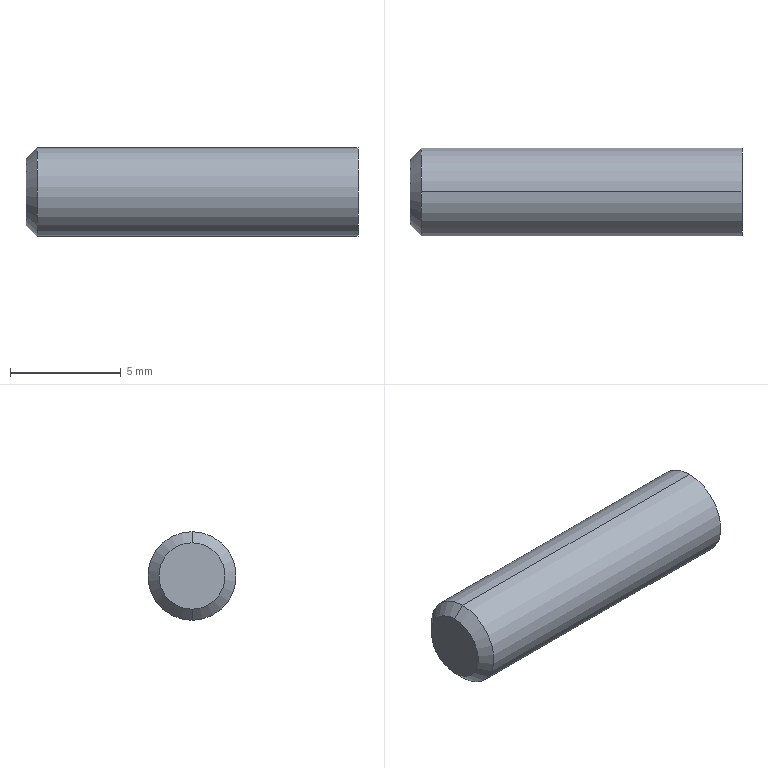Part | STEP file | 1 solid | 6 faces | box 15 x 4 x 4 mm | volume 187.056 mm3 | cylinder 2 | cone 2 | plane 2 | commonest cylinder face diameters 4 x2
STEP:
#1=CARTESIAN_POINT('',(0.,0.,0.));
#2=DIRECTION('',(0.,0.,1.));
#3=DIRECTION('',(1.,0.,0.));
#4=AXIS2_PLACEMENT_3D('',#1,#2,#3);
#5=CARTESIAN_POINT('',(-516.273,4552.173,1399.094));
#6=VERTEX_POINT('',#5);
#7=CARTESIAN_POINT('',(-501.773,4552.173,1399.094));
#8=VERTEX_POINT('',#7);
#9=CARTESIAN_POINT('',(-516.273,4552.173,1399.094));
#10=DIRECTION('',(1.,0.,0.));
#11=VECTOR('',#10,1.);
#12=LINE('',#9,#11);
#13=CARTESIAN_POINT('',(-513.773,4552.173,1397.094));
#14=DIRECTION('',(1.,0.,0.));
#15=DIRECTION('',(0.,0.,-1.));
#16=AXIS2_PLACEMENT_3D('',#13,#14,#15);
#17=CYLINDRICAL_SURFACE('',#16,2.);
#18=CARTESIAN_POINT('',(3.142,-2.5));
#19=DIRECTION('',(0.,1.));
#20=VECTOR('',#19,1.);
#21=LINE('',#18,#20);
#22=(GEOMETRIC_REPRESENTATION_CONTEXT(2)PARAMETRIC_REPRESENTATION_CONTEXT()REPRESENTATION_CONTEXT('',''));
#23=DEFINITIONAL_REPRESENTATION('',(#21),#22);
#24=PCURVE('',#17,#23);
#25=CARTESIAN_POINT('',(-513.773,4552.173,1397.094));
#26=DIRECTION('',(1.,0.,0.));
#27=DIRECTION('',(0.,0.,-1.));
#28=AXIS2_PLACEMENT_3D('',#25,#26,#27);
#29=CYLINDRICAL_SURFACE('',#28,2.);
#30=CARTESIAN_POINT('',(3.142,-2.5));
#31=DIRECTION('',(0.,1.));
#32=VECTOR('',#31,1.);
#33=LINE('',#30,#32);
#34=(GEOMETRIC_REPRESENTATION_CONTEXT(2)PARAMETRIC_REPRESENTATION_CONTEXT()REPRESENTATION_CONTEXT('',''));
#35=DEFINITIONAL_REPRESENTATION('',(#33),#34);
#36=PCURVE('',#29,#35);
#37=SURFACE_CURVE('',#12,(#24,#36),.PCURVE_S1.);
#38=EDGE_CURVE('',#6,#8,#37,.T.);
#39=ORIENTED_EDGE('',*,*,#38,.T.);
#40=CARTESIAN_POINT('',(-501.773,4552.173,1395.094));
#41=VERTEX_POINT('',#40);
#42=CARTESIAN_POINT('',(-501.773,4552.173,1397.094));
#43=DIRECTION('',(1.,0.,0.));
#44=DIRECTION('',(0.,0.,-1.));
#45=AXIS2_PLACEMENT_3D('',#42,#43,#44);
#46=CIRCLE('',#45,2.);
#47=CARTESIAN_POINT('',(0.,12.));
#48=DIRECTION('',(1.,0.));
#49=VECTOR('',#48,1.);
#50=LINE('',#47,#49);
#51=(GEOMETRIC_REPRESENTATION_CONTEXT(2)PARAMETRIC_REPRESENTATION_CONTEXT()REPRESENTATION_CONTEXT('',''));
#52=DEFINITIONAL_REPRESENTATION('',(#50),#51);
#53=PCURVE('',#17,#52);
#54=CARTESIAN_POINT('',(-501.773,4552.173,1397.094));
#55=DIRECTION('',(-1.,0.,0.));
#56=DIRECTION('',(0.,0.,1.));
#57=AXIS2_PLACEMENT_3D('',#54,#55,#56);
#58=PLANE('',#57);
#59=CARTESIAN_POINT('',(-2.,0.));
#60=CARTESIAN_POINT('',(-2.,3.464));
#61=CARTESIAN_POINT('',(1.,1.732));
#62=CARTESIAN_POINT('',(4.,0.));
#63=CARTESIAN_POINT('',(1.,-1.732));
#64=CARTESIAN_POINT('',(-2.,-3.464));
#65=CARTESIAN_POINT('',(-2.,0.));
#66=(BOUNDED_CURVE()B_SPLINE_CURVE(2,(#59,#60,#61,#62,#63,#64,#65),.UNSPECIFIED.,.T.,.F.)B_SPLINE_CURVE_WITH_KNOTS((1,2,2,2,2,1),(-2.094,0.,2.094,4.189,6.283,8.378),.UNSPECIFIED.)CURVE()GEOMETRIC_REPRESENTATION_ITEM()RATIONAL_B_SPLINE_CURVE((1.,0.5,1.,0.5,1.,0.5,1.))REPRESENTATION_ITEM(''));
#67=(GEOMETRIC_REPRESENTATION_CONTEXT(2)PARAMETRIC_REPRESENTATION_CONTEXT()REPRESENTATION_CONTEXT('',''));
#68=DEFINITIONAL_REPRESENTATION('',(#66),#67);
#69=PCURVE('',#58,#68);
#70=SURFACE_CURVE('',#46,(#53,#69),.PCURVE_S1.);
#71=EDGE_CURVE('',#41,#8,#70,.T.);
#72=ORIENTED_EDGE('',*,*,#71,.F.);
#73=CARTESIAN_POINT('',(-516.273,4552.173,1395.094));
#74=VERTEX_POINT('',#73);
#75=CARTESIAN_POINT('',(-516.273,4552.173,1395.094));
#76=DIRECTION('',(1.,0.,0.));
#77=VECTOR('',#76,1.);
#78=LINE('',#75,#77);
#79=CARTESIAN_POINT('',(0.,-2.5));
#80=DIRECTION('',(0.,1.));
#81=VECTOR('',#80,1.);
#82=LINE('',#79,#81);
#83=(GEOMETRIC_REPRESENTATION_CONTEXT(2)PARAMETRIC_REPRESENTATION_CONTEXT()REPRESENTATION_CONTEXT('',''));
#84=DEFINITIONAL_REPRESENTATION('',(#82),#83);
#85=PCURVE('',#17,#84);
#86=CARTESIAN_POINT('',(6.283,-2.5));
#87=DIRECTION('',(0.,1.));
#88=VECTOR('',#87,1.);
#89=LINE('',#86,#88);
#90=(GEOMETRIC_REPRESENTATION_CONTEXT(2)PARAMETRIC_REPRESENTATION_CONTEXT()REPRESENTATION_CONTEXT('',''));
#91=DEFINITIONAL_REPRESENTATION('',(#89),#90);
#92=PCURVE('',#29,#91);
#93=SURFACE_CURVE('',#78,(#85,#92),.PCURVE_S1.);
#94=EDGE_CURVE('',#74,#41,#93,.T.);
#95=ORIENTED_EDGE('',*,*,#94,.F.);
#96=CARTESIAN_POINT('',(-516.273,4552.173,1397.094));
#97=DIRECTION('',(-1.,0.,0.));
#98=DIRECTION('',(0.,0.,1.));
#99=AXIS2_PLACEMENT_3D('',#96,#97,#98);
#100=CIRCLE('',#99,2.);
#101=CARTESIAN_POINT('',(3.142,-2.5));
#102=DIRECTION('',(-1.,0.));
#103=VECTOR('',#102,1.);
#104=LINE('',#101,#103);
#105=(GEOMETRIC_REPRESENTATION_CONTEXT(2)PARAMETRIC_REPRESENTATION_CONTEXT()REPRESENTATION_CONTEXT('',''));
#106=DEFINITIONAL_REPRESENTATION('',(#104),#105);
#107=PCURVE('',#17,#106);
#108=CARTESIAN_POINT('',(-516.523,4552.173,1397.094));
#109=DIRECTION('',(1.,0.,0.));
#110=DIRECTION('',(0.,0.,-1.));
#111=AXIS2_PLACEMENT_3D('',#108,#109,#110);
#112=CONICAL_SURFACE('',#111,1.75,0.7854);
#113=CARTESIAN_POINT('',(3.142,0.25));
#114=DIRECTION('',(-1.,0.));
#115=VECTOR('',#114,1.);
#116=LINE('',#113,#115);
#117=(GEOMETRIC_REPRESENTATION_CONTEXT(2)PARAMETRIC_REPRESENTATION_CONTEXT()REPRESENTATION_CONTEXT('',''));
#118=DEFINITIONAL_REPRESENTATION('',(#116),#117);
#119=PCURVE('',#112,#118);
#120=SURFACE_CURVE('',#100,(#107,#119),.PCURVE_S1.);
#121=EDGE_CURVE('',#6,#74,#120,.T.);
#122=ORIENTED_EDGE('',*,*,#121,.F.);
#123=EDGE_LOOP('',(#39,#72,#95,#122));
#124=FACE_BOUND('',#123,.T.);
#125=ADVANCED_FACE('',(#124),#17,.T.);
#126=CARTESIAN_POINT('',(-516.773,4552.173,1395.594));
#127=VERTEX_POINT('',#126);
#128=CARTESIAN_POINT('',(-516.773,4552.173,1395.594));
#129=DIRECTION('',(0.7071,0.,-0.7071));
#130=VECTOR('',#129,1.);
#131=LINE('',#128,#130);
#132=CARTESIAN_POINT('',(0.,-0.25));
#133=DIRECTION('',(0.,1.));
#134=VECTOR('',#133,1.);
#135=LINE('',#132,#134);
#136=(GEOMETRIC_REPRESENTATION_CONTEXT(2)PARAMETRIC_REPRESENTATION_CONTEXT()REPRESENTATION_CONTEXT('',''));
#137=DEFINITIONAL_REPRESENTATION('',(#135),#136);
#138=PCURVE('',#112,#137);
#139=CARTESIAN_POINT('',(-516.523,4552.173,1397.094));
#140=DIRECTION('',(1.,0.,0.));
#141=DIRECTION('',(0.,0.,-1.));
#142=AXIS2_PLACEMENT_3D('',#139,#140,#141);
#143=CONICAL_SURFACE('',#142,1.75,0.7854);
#144=CARTESIAN_POINT('',(6.283,-0.25));
#145=DIRECTION('',(0.,1.));
#146=VECTOR('',#145,1.);
#147=LINE('',#144,#146);
#148=(GEOMETRIC_REPRESENTATION_CONTEXT(2)PARAMETRIC_REPRESENTATION_CONTEXT()REPRESENTATION_CONTEXT('',''));
#149=DEFINITIONAL_REPRESENTATION('',(#147),#148);
#150=PCURVE('',#143,#149);
#151=SURFACE_CURVE('',#131,(#138,#150),.PCURVE_S1.);
#152=EDGE_CURVE('',#127,#74,#151,.T.);
#153=ORIENTED_EDGE('',*,*,#152,.F.);
#154=CARTESIAN_POINT('',(-516.773,4552.173,1398.594));
#155=VERTEX_POINT('',#154);
#156=CARTESIAN_POINT('',(-516.773,4552.173,1397.094));
#157=DIRECTION('',(-1.,0.,0.));
#158=DIRECTION('',(0.,0.,1.));
#159=AXIS2_PLACEMENT_3D('',#156,#157,#158);
#160=CIRCLE('',#159,1.5);
#161=CARTESIAN_POINT('',(3.142,-0.25));
#162=DIRECTION('',(-1.,0.));
#163=VECTOR('',#162,1.);
#164=LINE('',#161,#163);
#165=(GEOMETRIC_REPRESENTATION_CONTEXT(2)PARAMETRIC_REPRESENTATION_CONTEXT()REPRESENTATION_CONTEXT('',''));
#166=DEFINITIONAL_REPRESENTATION('',(#164),#165);
#167=PCURVE('',#112,#166);
#168=CARTESIAN_POINT('',(-516.773,4552.173,1397.094));
#169=DIRECTION('',(-1.,0.,0.));
#170=DIRECTION('',(0.,0.,1.));
#171=AXIS2_PLACEMENT_3D('',#168,#169,#170);
#172=PLANE('',#171);
#173=CARTESIAN_POINT('',(0.,0.));
#174=DIRECTION('',(1.,0.));
#175=AXIS2_PLACEMENT_2D('',#173,#174);
#176=CIRCLE('',#175,1.5);
#177=(GEOMETRIC_REPRESENTATION_CONTEXT(2)PARAMETRIC_REPRESENTATION_CONTEXT()REPRESENTATION_CONTEXT('',''));
#178=DEFINITIONAL_REPRESENTATION('',(#176),#177);
#179=PCURVE('',#172,#178);
#180=SURFACE_CURVE('',#160,(#167,#179),.PCURVE_S1.);
#181=EDGE_CURVE('',#155,#127,#180,.T.);
#182=ORIENTED_EDGE('',*,*,#181,.F.);
#183=CARTESIAN_POINT('',(-516.773,4552.173,1398.594));
#184=DIRECTION('',(0.7071,0.,0.7071));
#185=VECTOR('',#184,1.);
#186=LINE('',#183,#185);
#187=CARTESIAN_POINT('',(3.142,-0.25));
#188=DIRECTION('',(0.,1.));
#189=VECTOR('',#188,1.);
#190=LINE('',#187,#189);
#191=(GEOMETRIC_REPRESENTATION_CONTEXT(2)PARAMETRIC_REPRESENTATION_CONTEXT()REPRESENTATION_CONTEXT('',''));
#192=DEFINITIONAL_REPRESENTATION('',(#190),#191);
#193=PCURVE('',#112,#192);
#194=CARTESIAN_POINT('',(3.142,-0.25));
#195=DIRECTION('',(0.,1.));
#196=VECTOR('',#195,1.);
#197=LINE('',#194,#196);
#198=(GEOMETRIC_REPRESENTATION_CONTEXT(2)PARAMETRIC_REPRESENTATION_CONTEXT()REPRESENTATION_CONTEXT('',''));
#199=DEFINITIONAL_REPRESENTATION('',(#197),#198);
#200=PCURVE('',#143,#199);
#201=SURFACE_CURVE('',#186,(#193,#200),.PCURVE_S1.);
#202=EDGE_CURVE('',#155,#6,#201,.T.);
#203=ORIENTED_EDGE('',*,*,#202,.T.);
#204=ORIENTED_EDGE('',*,*,#121,.T.);
#205=EDGE_LOOP('',(#153,#182,#203,#204));
#206=FACE_BOUND('',#205,.T.);
#207=ADVANCED_FACE('',(#206),#112,.T.);
#208=ORIENTED_EDGE('',*,*,#202,.F.);
#209=CARTESIAN_POINT('',(-516.773,4552.173,1397.094));
#210=DIRECTION('',(-1.,0.,0.));
#211=DIRECTION('',(0.,0.,-1.));
#212=AXIS2_PLACEMENT_3D('',#209,#210,#211);
#213=CIRCLE('',#212,1.5);
#214=CARTESIAN_POINT('',(6.283,-0.25));
#215=DIRECTION('',(-1.,0.));
#216=VECTOR('',#215,1.);
#217=LINE('',#214,#216);
#218=(GEOMETRIC_REPRESENTATION_CONTEXT(2)PARAMETRIC_REPRESENTATION_CONTEXT()REPRESENTATION_CONTEXT('',''));
#219=DEFINITIONAL_REPRESENTATION('',(#217),#218);
#220=PCURVE('',#143,#219);
#221=CARTESIAN_POINT('',(0.,0.));
#222=DIRECTION('',(-1.,0.));
#223=AXIS2_PLACEMENT_2D('',#221,#222);
#224=CIRCLE('',#223,1.5);
#225=(GEOMETRIC_REPRESENTATION_CONTEXT(2)PARAMETRIC_REPRESENTATION_CONTEXT()REPRESENTATION_CONTEXT('',''));
#226=DEFINITIONAL_REPRESENTATION('',(#224),#225);
#227=PCURVE('',#172,#226);
#228=SURFACE_CURVE('',#213,(#220,#227),.PCURVE_S1.);
#229=EDGE_CURVE('',#127,#155,#228,.T.);
#230=ORIENTED_EDGE('',*,*,#229,.F.);
#231=ORIENTED_EDGE('',*,*,#152,.T.);
#232=CARTESIAN_POINT('',(-516.273,4552.173,1397.094));
#233=DIRECTION('',(-1.,0.,0.));
#234=DIRECTION('',(0.,0.,-1.));
#235=AXIS2_PLACEMENT_3D('',#232,#233,#234);
#236=CIRCLE('',#235,2.);
#237=CARTESIAN_POINT('',(6.283,0.25));
#238=DIRECTION('',(-1.,0.));
#239=VECTOR('',#238,1.);
#240=LINE('',#237,#239);
#241=(GEOMETRIC_REPRESENTATION_CONTEXT(2)PARAMETRIC_REPRESENTATION_CONTEXT()REPRESENTATION_CONTEXT('',''));
#242=DEFINITIONAL_REPRESENTATION('',(#240),#241);
#243=PCURVE('',#143,#242);
#244=CARTESIAN_POINT('',(6.283,-2.5));
#245=DIRECTION('',(-1.,0.));
#246=VECTOR('',#245,1.);
#247=LINE('',#244,#246);
#248=(GEOMETRIC_REPRESENTATION_CONTEXT(2)PARAMETRIC_REPRESENTATION_CONTEXT()REPRESENTATION_CONTEXT('',''));
#249=DEFINITIONAL_REPRESENTATION('',(#247),#248);
#250=PCURVE('',#29,#249);
#251=SURFACE_CURVE('',#236,(#243,#250),.PCURVE_S1.);
#252=EDGE_CURVE('',#74,#6,#251,.T.);
#253=ORIENTED_EDGE('',*,*,#252,.T.);
#254=EDGE_LOOP('',(#208,#230,#231,#253));
#255=FACE_BOUND('',#254,.T.);
#256=ADVANCED_FACE('',(#255),#143,.T.);
#257=ORIENTED_EDGE('',*,*,#94,.T.);
#258=CARTESIAN_POINT('',(-501.773,4552.173,1397.094));
#259=DIRECTION('',(1.,0.,0.));
#260=DIRECTION('',(0.,0.,1.));
#261=AXIS2_PLACEMENT_3D('',#258,#259,#260);
#262=CIRCLE('',#261,2.);
#263=CARTESIAN_POINT('',(3.142,12.));
#264=DIRECTION('',(1.,0.));
#265=VECTOR('',#264,1.);
#266=LINE('',#263,#265);
#267=(GEOMETRIC_REPRESENTATION_CONTEXT(2)PARAMETRIC_REPRESENTATION_CONTEXT()REPRESENTATION_CONTEXT('',''));
#268=DEFINITIONAL_REPRESENTATION('',(#266),#267);
#269=PCURVE('',#29,#268);
#270=CARTESIAN_POINT('',(2.,0.));
#271=CARTESIAN_POINT('',(2.,-3.464));
#272=CARTESIAN_POINT('',(-1.,-1.732));
#273=CARTESIAN_POINT('',(-4.,0.));
#274=CARTESIAN_POINT('',(-1.,1.732));
#275=CARTESIAN_POINT('',(2.,3.464));
#276=CARTESIAN_POINT('',(2.,0.));
#277=(BOUNDED_CURVE()B_SPLINE_CURVE(2,(#270,#271,#272,#273,#274,#275,#276),.UNSPECIFIED.,.T.,.F.)B_SPLINE_CURVE_WITH_KNOTS((1,2,2,2,2,1),(-2.094,0.,2.094,4.189,6.283,8.378),.UNSPECIFIED.)CURVE()GEOMETRIC_REPRESENTATION_ITEM()RATIONAL_B_SPLINE_CURVE((1.,0.5,1.,0.5,1.,0.5,1.))REPRESENTATION_ITEM(''));
#278=(GEOMETRIC_REPRESENTATION_CONTEXT(2)PARAMETRIC_REPRESENTATION_CONTEXT()REPRESENTATION_CONTEXT('',''));
#279=DEFINITIONAL_REPRESENTATION('',(#277),#278);
#280=PCURVE('',#58,#279);
#281=SURFACE_CURVE('',#262,(#269,#280),.PCURVE_S1.);
#282=EDGE_CURVE('',#8,#41,#281,.T.);
#283=ORIENTED_EDGE('',*,*,#282,.F.);
#284=ORIENTED_EDGE('',*,*,#38,.F.);
#285=ORIENTED_EDGE('',*,*,#252,.F.);
#286=EDGE_LOOP('',(#257,#283,#284,#285));
#287=FACE_BOUND('',#286,.T.);
#288=ADVANCED_FACE('',(#287),#29,.T.);
#289=ORIENTED_EDGE('',*,*,#282,.F.);
#290=ORIENTED_EDGE('',*,*,#71,.F.);
#291=EDGE_LOOP('',(#289,#290));
#292=FACE_BOUND('',#291,.F.);
#293=ADVANCED_FACE('',(#292),#58,.F.);
#294=ORIENTED_EDGE('',*,*,#181,.F.);
#295=ORIENTED_EDGE('',*,*,#229,.F.);
#296=EDGE_LOOP('',(#294,#295));
#297=FACE_BOUND('',#296,.F.);
#298=ADVANCED_FACE('',(#297),#172,.T.);
#299=CLOSED_SHELL('',(#125,#207,#256,#288,#293,#298));
#300=MANIFOLD_SOLID_BREP('',#299);
#301=(LENGTH_UNIT()NAMED_UNIT(*)SI_UNIT(.MILLI.,.METRE.));
#302=UNCERTAINTY_MEASURE_WITH_UNIT(LENGTH_MEASURE(0.0000001),#301,'','');
#303=(NAMED_UNIT(*)PLANE_ANGLE_UNIT()SI_UNIT($,.RADIAN.));
#304=(NAMED_UNIT(*)SI_UNIT($,.STERADIAN.)SOLID_ANGLE_UNIT());
#305=(GEOMETRIC_REPRESENTATION_CONTEXT(3)GLOBAL_UNCERTAINTY_ASSIGNED_CONTEXT((#302))GLOBAL_UNIT_ASSIGNED_CONTEXT((#301,#303,#304))REPRESENTATION_CONTEXT('',''));
#306=ADVANCED_BREP_SHAPE_REPRESENTATION('',(#4,#300),#305);